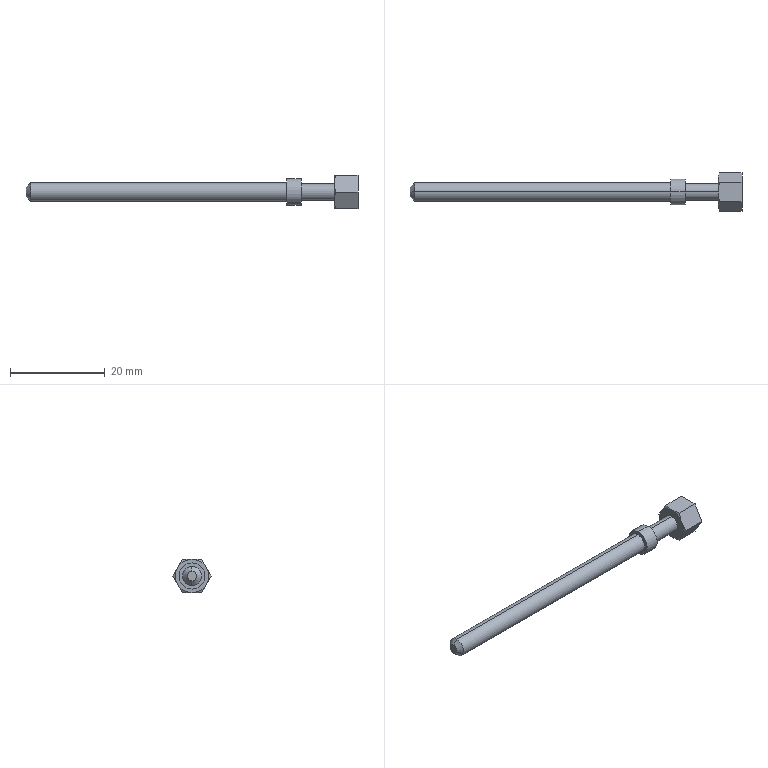Part | STEP file | 11-AJST4-5511 | 1 solid | 25 faces | box 70 x 8.083 x 7 mm | volume 1036 mm3 | plane 11 | cone 8 | cylinder 6 | commonest cylinder face diameters 3.5 x2 4 x2 5.5 x2
STEP:
#1=CARTESIAN_POINT('',(0.,0.,1.));
#2=VERTEX_POINT('',#1);
#3=CARTESIAN_POINT('',(0.,0.,-1.));
#4=VERTEX_POINT('',#3);
#5=CARTESIAN_POINT('',(0.,0.,0.));
#6=DIRECTION('',(-1.,0.,0.));
#7=DIRECTION('',(0.,0.,-1.));
#8=AXIS2_PLACEMENT_3D('',#5,#6,#7);
#9=CIRCLE('',#8,1.);
#10=EDGE_CURVE('',#2,#4,#9,.T.);
#11=ORIENTED_EDGE('',*,*,#10,.F.);
#12=CARTESIAN_POINT('',(1.,0.,2.));
#13=VERTEX_POINT('',#12);
#14=CARTESIAN_POINT('',(0.,0.,1.));
#15=DIRECTION('',(0.7071,0.,0.7071));
#16=VECTOR('',#15,1000.);
#17=LINE('',#14,#16);
#18=EDGE_CURVE('',#2,#13,#17,.T.);
#19=ORIENTED_EDGE('',*,*,#18,.T.);
#20=CARTESIAN_POINT('',(1.,0.,-2.));
#21=VERTEX_POINT('',#20);
#22=CARTESIAN_POINT('',(1.,0.,0.));
#23=DIRECTION('',(1.,0.,0.));
#24=DIRECTION('',(0.,0.,-1.));
#25=AXIS2_PLACEMENT_3D('',#22,#23,#24);
#26=CIRCLE('',#25,2.);
#27=EDGE_CURVE('',#21,#13,#26,.T.);
#28=ORIENTED_EDGE('',*,*,#27,.F.);
#29=CARTESIAN_POINT('',(0.,0.,-1.));
#30=DIRECTION('',(0.7071,0.,-0.7071));
#31=VECTOR('',#30,1000.);
#32=LINE('',#29,#31);
#33=EDGE_CURVE('',#4,#21,#32,.T.);
#34=ORIENTED_EDGE('',*,*,#33,.F.);
#35=EDGE_LOOP('',(#11,#19,#28,#34));
#36=FACE_OUTER_BOUND('',#35,.T.);
#37=CARTESIAN_POINT('',(0.,0.,0.));
#38=DIRECTION('',(1.,0.,0.));
#39=DIRECTION('',(0.,0.,-1.));
#40=AXIS2_PLACEMENT_3D('',#37,#38,#39);
#41=CONICAL_SURFACE('',#40,1.,0.7854);
#42=ADVANCED_FACE('',(#36),#41,.T.);
#43=CARTESIAN_POINT('',(65.,0.,-1.75));
#44=VERTEX_POINT('',#43);
#45=CARTESIAN_POINT('',(65.,0.,1.75));
#46=VERTEX_POINT('',#45);
#47=CARTESIAN_POINT('',(65.,0.,0.));
#48=DIRECTION('',(1.,0.,0.));
#49=DIRECTION('',(0.,0.,-1.));
#50=AXIS2_PLACEMENT_3D('',#47,#48,#49);
#51=CIRCLE('',#50,1.75);
#52=EDGE_CURVE('',#44,#46,#51,.T.);
#53=ORIENTED_EDGE('',*,*,#52,.F.);
#54=CARTESIAN_POINT('',(58.,0.,-1.75));
#55=VERTEX_POINT('',#54);
#56=CARTESIAN_POINT('',(0.,0.,-1.75));
#57=DIRECTION('',(-1.,0.,0.));
#58=VECTOR('',#57,1000.);
#59=LINE('',#56,#58);
#60=EDGE_CURVE('',#44,#55,#59,.T.);
#61=ORIENTED_EDGE('',*,*,#60,.T.);
#62=CARTESIAN_POINT('',(58.,0.,1.75));
#63=VERTEX_POINT('',#62);
#64=CARTESIAN_POINT('',(58.,0.,0.));
#65=DIRECTION('',(-1.,0.,0.));
#66=DIRECTION('',(0.,0.,1.));
#67=AXIS2_PLACEMENT_3D('',#64,#65,#66);
#68=CIRCLE('',#67,1.75);
#69=EDGE_CURVE('',#63,#55,#68,.T.);
#70=ORIENTED_EDGE('',*,*,#69,.F.);
#71=CARTESIAN_POINT('',(0.,0.,1.75));
#72=DIRECTION('',(-1.,0.,0.));
#73=VECTOR('',#72,1000.);
#74=LINE('',#71,#73);
#75=EDGE_CURVE('',#46,#63,#74,.T.);
#76=ORIENTED_EDGE('',*,*,#75,.F.);
#77=EDGE_LOOP('',(#53,#61,#70,#76));
#78=FACE_OUTER_BOUND('',#77,.T.);
#79=CARTESIAN_POINT('',(0.,0.,0.));
#80=DIRECTION('',(-1.,0.,0.));
#81=DIRECTION('',(0.,0.,1.));
#82=AXIS2_PLACEMENT_3D('',#79,#80,#81);
#83=CYLINDRICAL_SURFACE('',#82,1.75);
#84=ADVANCED_FACE('',(#78),#83,.T.);
#85=CARTESIAN_POINT('',(58.,0.,2.75));
#86=VERTEX_POINT('',#85);
#87=CARTESIAN_POINT('',(58.,0.,-2.75));
#88=VERTEX_POINT('',#87);
#89=CARTESIAN_POINT('',(58.,0.,0.));
#90=DIRECTION('',(-1.,0.,0.));
#91=DIRECTION('',(0.,0.,1.));
#92=AXIS2_PLACEMENT_3D('',#89,#90,#91);
#93=CIRCLE('',#92,2.75);
#94=EDGE_CURVE('',#86,#88,#93,.T.);
#95=ORIENTED_EDGE('',*,*,#94,.T.);
#96=CARTESIAN_POINT('',(55.,0.,-2.75));
#97=VERTEX_POINT('',#96);
#98=CARTESIAN_POINT('',(0.,0.,-2.75));
#99=DIRECTION('',(-1.,0.,0.));
#100=VECTOR('',#99,1000.);
#101=LINE('',#98,#100);
#102=EDGE_CURVE('',#88,#97,#101,.T.);
#103=ORIENTED_EDGE('',*,*,#102,.T.);
#104=CARTESIAN_POINT('',(55.,0.,2.75));
#105=VERTEX_POINT('',#104);
#106=CARTESIAN_POINT('',(55.,0.,0.));
#107=DIRECTION('',(-1.,0.,0.));
#108=DIRECTION('',(0.,0.,1.));
#109=AXIS2_PLACEMENT_3D('',#106,#107,#108);
#110=CIRCLE('',#109,2.75);
#111=EDGE_CURVE('',#105,#97,#110,.T.);
#112=ORIENTED_EDGE('',*,*,#111,.F.);
#113=CARTESIAN_POINT('',(0.,0.,2.75));
#114=DIRECTION('',(-1.,0.,0.));
#115=VECTOR('',#114,1000.);
#116=LINE('',#113,#115);
#117=EDGE_CURVE('',#86,#105,#116,.T.);
#118=ORIENTED_EDGE('',*,*,#117,.F.);
#119=EDGE_LOOP('',(#95,#103,#112,#118));
#120=FACE_OUTER_BOUND('',#119,.T.);
#121=CARTESIAN_POINT('',(0.,0.,0.));
#122=DIRECTION('',(-1.,0.,0.));
#123=DIRECTION('',(0.,0.,1.));
#124=AXIS2_PLACEMENT_3D('',#121,#122,#123);
#125=CYLINDRICAL_SURFACE('',#124,2.75);
#126=ADVANCED_FACE('',(#120),#125,.T.);
#127=CARTESIAN_POINT('',(55.,0.,2.));
#128=VERTEX_POINT('',#127);
#129=CARTESIAN_POINT('',(55.,0.,-2.));
#130=VERTEX_POINT('',#129);
#131=CARTESIAN_POINT('',(55.,0.,0.));
#132=DIRECTION('',(-1.,0.,0.));
#133=DIRECTION('',(0.,0.,1.));
#134=AXIS2_PLACEMENT_3D('',#131,#132,#133);
#135=CIRCLE('',#134,2.);
#136=EDGE_CURVE('',#128,#130,#135,.T.);
#137=ORIENTED_EDGE('',*,*,#136,.T.);
#138=CARTESIAN_POINT('',(0.,0.,-2.));
#139=DIRECTION('',(-1.,0.,0.));
#140=VECTOR('',#139,1000.);
#141=LINE('',#138,#140);
#142=EDGE_CURVE('',#130,#21,#141,.T.);
#143=ORIENTED_EDGE('',*,*,#142,.T.);
#144=ORIENTED_EDGE('',*,*,#27,.T.);
#145=CARTESIAN_POINT('',(0.,0.,2.));
#146=DIRECTION('',(-1.,0.,0.));
#147=VECTOR('',#146,1000.);
#148=LINE('',#145,#147);
#149=EDGE_CURVE('',#128,#13,#148,.T.);
#150=ORIENTED_EDGE('',*,*,#149,.F.);
#151=EDGE_LOOP('',(#137,#143,#144,#150));
#152=FACE_OUTER_BOUND('',#151,.T.);
#153=CARTESIAN_POINT('',(0.,0.,0.));
#154=DIRECTION('',(-1.,0.,0.));
#155=DIRECTION('',(0.,0.,1.));
#156=AXIS2_PLACEMENT_3D('',#153,#154,#155);
#157=CYLINDRICAL_SURFACE('',#156,2.);
#158=ADVANCED_FACE('',(#152),#157,.T.);
#159=CARTESIAN_POINT('',(65.,0.,0.));
#160=DIRECTION('',(1.,0.,0.));
#161=DIRECTION('',(0.,0.,-1.));
#162=AXIS2_PLACEMENT_3D('',#159,#160,#161);
#163=CIRCLE('',#162,1.75);
#164=EDGE_CURVE('',#46,#44,#163,.T.);
#165=ORIENTED_EDGE('',*,*,#164,.T.);
#166=ORIENTED_EDGE('',*,*,#52,.T.);
#167=EDGE_LOOP('',(#165,#166));
#168=FACE_BOUND('',#167,.T.);
#169=CARTESIAN_POINT('',(65.,3.031,-1.75));
#170=VERTEX_POINT('',#169);
#171=CARTESIAN_POINT('',(65.,0.,-3.5));
#172=VERTEX_POINT('',#171);
#173=CARTESIAN_POINT('',(65.,0.,0.));
#174=DIRECTION('',(-1.,0.,0.));
#175=DIRECTION('',(0.,0.,1.));
#176=AXIS2_PLACEMENT_3D('',#173,#174,#175);
#177=CIRCLE('',#176,3.5);
#178=EDGE_CURVE('',#170,#172,#177,.T.);
#179=ORIENTED_EDGE('',*,*,#178,.T.);
#180=CARTESIAN_POINT('',(65.,-3.031,-1.75));
#181=VERTEX_POINT('',#180);
#182=CARTESIAN_POINT('',(65.,0.,0.));
#183=DIRECTION('',(-1.,0.,0.));
#184=DIRECTION('',(0.,0.,1.));
#185=AXIS2_PLACEMENT_3D('',#182,#183,#184);
#186=CIRCLE('',#185,3.5);
#187=EDGE_CURVE('',#172,#181,#186,.T.);
#188=ORIENTED_EDGE('',*,*,#187,.T.);
#189=CARTESIAN_POINT('',(65.,-3.031,1.75));
#190=VERTEX_POINT('',#189);
#191=CARTESIAN_POINT('',(65.,0.,0.));
#192=DIRECTION('',(-1.,0.,0.));
#193=DIRECTION('',(0.,0.,1.));
#194=AXIS2_PLACEMENT_3D('',#191,#192,#193);
#195=CIRCLE('',#194,3.5);
#196=EDGE_CURVE('',#181,#190,#195,.T.);
#197=ORIENTED_EDGE('',*,*,#196,.T.);
#198=CARTESIAN_POINT('',(65.,0.,3.5));
#199=VERTEX_POINT('',#198);
#200=CARTESIAN_POINT('',(65.,0.,0.));
#201=DIRECTION('',(-1.,0.,0.));
#202=DIRECTION('',(0.,0.,1.));
#203=AXIS2_PLACEMENT_3D('',#200,#201,#202);
#204=CIRCLE('',#203,3.5);
#205=EDGE_CURVE('',#190,#199,#204,.T.);
#206=ORIENTED_EDGE('',*,*,#205,.T.);
#207=CARTESIAN_POINT('',(65.,3.031,1.75));
#208=VERTEX_POINT('',#207);
#209=CARTESIAN_POINT('',(65.,0.,0.));
#210=DIRECTION('',(-1.,0.,0.));
#211=DIRECTION('',(0.,0.,1.));
#212=AXIS2_PLACEMENT_3D('',#209,#210,#211);
#213=CIRCLE('',#212,3.5);
#214=EDGE_CURVE('',#199,#208,#213,.T.);
#215=ORIENTED_EDGE('',*,*,#214,.T.);
#216=CARTESIAN_POINT('',(65.,0.,0.));
#217=DIRECTION('',(-1.,0.,0.));
#218=DIRECTION('',(0.,0.,1.));
#219=AXIS2_PLACEMENT_3D('',#216,#217,#218);
#220=CIRCLE('',#219,3.5);
#221=EDGE_CURVE('',#208,#170,#220,.T.);
#222=ORIENTED_EDGE('',*,*,#221,.T.);
#223=EDGE_LOOP('',(#179,#188,#197,#206,#215,#222));
#224=FACE_OUTER_BOUND('',#223,.T.);
#225=CARTESIAN_POINT('',(65.,0.,0.));
#226=DIRECTION('',(1.,0.,0.));
#227=DIRECTION('',(0.,0.,-1.));
#228=AXIS2_PLACEMENT_3D('',#225,#226,#227);
#229=PLANE('',#228);
#230=ADVANCED_FACE('',(#168,#224),#229,.F.);
#231=CARTESIAN_POINT('',(0.,0.,0.));
#232=DIRECTION('',(-1.,0.,0.));
#233=DIRECTION('',(0.,0.,-1.));
#234=AXIS2_PLACEMENT_3D('',#231,#232,#233);
#235=CIRCLE('',#234,1.);
#236=EDGE_CURVE('',#4,#2,#235,.T.);
#237=ORIENTED_EDGE('',*,*,#236,.T.);
#238=ORIENTED_EDGE('',*,*,#10,.T.);
#239=EDGE_LOOP('',(#237,#238));
#240=FACE_OUTER_BOUND('',#239,.T.);
#241=CARTESIAN_POINT('',(0.,0.,0.));
#242=DIRECTION('',(1.,0.,0.));
#243=DIRECTION('',(0.,0.,-1.));
#244=AXIS2_PLACEMENT_3D('',#241,#242,#243);
#245=PLANE('',#244);
#246=ADVANCED_FACE('',(#240),#245,.F.);
#247=ORIENTED_EDGE('',*,*,#142,.F.);
#248=CARTESIAN_POINT('',(55.,0.,0.));
#249=DIRECTION('',(-1.,0.,0.));
#250=DIRECTION('',(0.,0.,1.));
#251=AXIS2_PLACEMENT_3D('',#248,#249,#250);
#252=CIRCLE('',#251,2.);
#253=EDGE_CURVE('',#130,#128,#252,.T.);
#254=ORIENTED_EDGE('',*,*,#253,.T.);
#255=ORIENTED_EDGE('',*,*,#149,.T.);
#256=CARTESIAN_POINT('',(1.,0.,0.));
#257=DIRECTION('',(1.,0.,0.));
#258=DIRECTION('',(0.,0.,-1.));
#259=AXIS2_PLACEMENT_3D('',#256,#257,#258);
#260=CIRCLE('',#259,2.);
#261=EDGE_CURVE('',#13,#21,#260,.T.);
#262=ORIENTED_EDGE('',*,*,#261,.T.);
#263=EDGE_LOOP('',(#247,#254,#255,#262));
#264=FACE_OUTER_BOUND('',#263,.T.);
#265=CARTESIAN_POINT('',(0.,0.,0.));
#266=DIRECTION('',(-1.,0.,0.));
#267=DIRECTION('',(0.,0.,1.));
#268=AXIS2_PLACEMENT_3D('',#265,#266,#267);
#269=CYLINDRICAL_SURFACE('',#268,2.);
#270=ADVANCED_FACE('',(#264),#269,.T.);
#271=ORIENTED_EDGE('',*,*,#136,.F.);
#272=ORIENTED_EDGE('',*,*,#253,.F.);
#273=EDGE_LOOP('',(#271,#272));
#274=FACE_BOUND('',#273,.T.);
#275=ORIENTED_EDGE('',*,*,#111,.T.);
#276=CARTESIAN_POINT('',(55.,0.,0.));
#277=DIRECTION('',(-1.,0.,0.));
#278=DIRECTION('',(0.,0.,1.));
#279=AXIS2_PLACEMENT_3D('',#276,#277,#278);
#280=CIRCLE('',#279,2.75);
#281=EDGE_CURVE('',#97,#105,#280,.T.);
#282=ORIENTED_EDGE('',*,*,#281,.T.);
#283=EDGE_LOOP('',(#275,#282));
#284=FACE_OUTER_BOUND('',#283,.T.);
#285=CARTESIAN_POINT('',(55.,2.,0.));
#286=DIRECTION('',(1.,0.,0.));
#287=DIRECTION('',(0.,0.,-1.));
#288=AXIS2_PLACEMENT_3D('',#285,#286,#287);
#289=PLANE('',#288);
#290=ADVANCED_FACE('',(#274,#284),#289,.F.);
#291=ORIENTED_EDGE('',*,*,#102,.F.);
#292=CARTESIAN_POINT('',(58.,0.,0.));
#293=DIRECTION('',(-1.,0.,0.));
#294=DIRECTION('',(0.,0.,1.));
#295=AXIS2_PLACEMENT_3D('',#292,#293,#294);
#296=CIRCLE('',#295,2.75);
#297=EDGE_CURVE('',#88,#86,#296,.T.);
#298=ORIENTED_EDGE('',*,*,#297,.T.);
#299=ORIENTED_EDGE('',*,*,#117,.T.);
#300=ORIENTED_EDGE('',*,*,#281,.F.);
#301=EDGE_LOOP('',(#291,#298,#299,#300));
#302=FACE_OUTER_BOUND('',#301,.T.);
#303=CARTESIAN_POINT('',(0.,0.,0.));
#304=DIRECTION('',(-1.,0.,0.));
#305=DIRECTION('',(0.,0.,1.));
#306=AXIS2_PLACEMENT_3D('',#303,#304,#305);
#307=CYLINDRICAL_SURFACE('',#306,2.75);
#308=ADVANCED_FACE('',(#302),#307,.T.);
#309=ORIENTED_EDGE('',*,*,#94,.F.);
#310=ORIENTED_EDGE('',*,*,#297,.F.);
#311=EDGE_LOOP('',(#309,#310));
#312=FACE_OUTER_BOUND('',#311,.T.);
#313=ORIENTED_EDGE('',*,*,#69,.T.);
#314=CARTESIAN_POINT('',(58.,0.,0.));
#315=DIRECTION('',(-1.,0.,0.));
#316=DIRECTION('',(0.,0.,1.));
#317=AXIS2_PLACEMENT_3D('',#314,#315,#316);
#318=CIRCLE('',#317,1.75);
#319=EDGE_CURVE('',#55,#63,#318,.T.);
#320=ORIENTED_EDGE('',*,*,#319,.T.);
#321=EDGE_LOOP('',(#313,#320));
#322=FACE_BOUND('',#321,.T.);
#323=CARTESIAN_POINT('',(58.,2.75,0.));
#324=DIRECTION('',(-1.,0.,0.));
#325=DIRECTION('',(0.,0.,1.));
#326=AXIS2_PLACEMENT_3D('',#323,#324,#325);
#327=PLANE('',#326);
#328=ADVANCED_FACE('',(#312,#322),#327,.F.);
#329=ORIENTED_EDGE('',*,*,#60,.F.);
#330=ORIENTED_EDGE('',*,*,#164,.F.);
#331=ORIENTED_EDGE('',*,*,#75,.T.);
#332=ORIENTED_EDGE('',*,*,#319,.F.);
#333=EDGE_LOOP('',(#329,#330,#331,#332));
#334=FACE_OUTER_BOUND('',#333,.T.);
#335=CARTESIAN_POINT('',(0.,0.,0.));
#336=DIRECTION('',(-1.,0.,0.));
#337=DIRECTION('',(0.,0.,1.));
#338=AXIS2_PLACEMENT_3D('',#335,#336,#337);
#339=CYLINDRICAL_SURFACE('',#338,1.75);
#340=ADVANCED_FACE('',(#334),#339,.T.);
#341=CARTESIAN_POINT('',(65.313,-2.021,3.5));
#342=VERTEX_POINT('',#341);
#343=CARTESIAN_POINT('',(65.313,-2.021,3.5));
#344=CARTESIAN_POINT('',(65.218,-1.692,3.5));
#345=CARTESIAN_POINT('',(65.138,-1.355,3.5));
#346=CARTESIAN_POINT('',(65.029,-0.6807,3.5));
#347=CARTESIAN_POINT('',(65.,-0.3415,3.5));
#348=CARTESIAN_POINT('',(65.,0.,3.5));
#349=B_SPLINE_CURVE_WITH_KNOTS('',3,(#343,#344,#345,#346,#347,#348),.UNSPECIFIED.,.F.,.F.,(4,2,4),(0.003605,0.004627,0.005649),.UNSPECIFIED.);
#350=EDGE_CURVE('',#342,#199,#349,.T.);
#351=ORIENTED_EDGE('',*,*,#350,.T.);
#352=ORIENTED_EDGE('',*,*,#205,.F.);
#353=CARTESIAN_POINT('',(65.,-3.031,1.75));
#354=CARTESIAN_POINT('',(65.,-2.86,2.047));
#355=CARTESIAN_POINT('',(65.03,-2.688,2.344));
#356=CARTESIAN_POINT('',(65.139,-2.352,2.926));
#357=CARTESIAN_POINT('',(65.217,-2.186,3.214));
#358=CARTESIAN_POINT('',(65.313,-2.021,3.5));
#359=B_SPLINE_CURVE_WITH_KNOTS('',3,(#353,#354,#355,#356,#357,#358),.UNSPECIFIED.,.F.,.F.,(4,2,4),(0.002045,0.003063,0.004082),.UNSPECIFIED.);
#360=EDGE_CURVE('',#190,#342,#359,.T.);
#361=ORIENTED_EDGE('',*,*,#360,.T.);
#362=EDGE_LOOP('',(#351,#352,#361));
#363=FACE_OUTER_BOUND('',#362,.T.);
#364=CARTESIAN_POINT('',(65.,0.,0.));
#365=DIRECTION('',(1.,0.,0.));
#366=DIRECTION('',(0.,0.,-1.));
#367=AXIS2_PLACEMENT_3D('',#364,#365,#366);
#368=CONICAL_SURFACE('',#367,3.5,1.047);
#369=ADVANCED_FACE('',(#363),#368,.T.);
#370=CARTESIAN_POINT('',(65.313,-4.041,0.));
#371=VERTEX_POINT('',#370);
#372=CARTESIAN_POINT('',(65.,-3.031,-1.75));
#373=CARTESIAN_POINT('',(65.,-3.203,-1.453));
#374=CARTESIAN_POINT('',(65.03,-3.374,-1.156));
#375=CARTESIAN_POINT('',(65.139,-3.71,-0.5735));
#376=CARTESIAN_POINT('',(65.217,-3.877,-0.2856));
#377=CARTESIAN_POINT('',(65.313,-4.041,0.));
#378=B_SPLINE_CURVE_WITH_KNOTS('',3,(#372,#373,#374,#375,#376,#377),.UNSPECIFIED.,.F.,.F.,(4,2,4),(0.002045,0.003063,0.004082),.UNSPECIFIED.);
#379=EDGE_CURVE('',#181,#371,#378,.T.);
#380=ORIENTED_EDGE('',*,*,#379,.T.);
#381=CARTESIAN_POINT('',(65.313,-4.041,0.));
#382=CARTESIAN_POINT('',(65.122,-3.711,0.5726));
#383=CARTESIAN_POINT('',(65.,-3.375,1.154));
#384=CARTESIAN_POINT('',(65.,-3.031,1.75));
#385=B_SPLINE_CURVE_WITH_KNOTS('',3,(#381,#382,#383,#384),.UNSPECIFIED.,.F.,.F.,(4,4),(0.000000238,0.002045),.UNSPECIFIED.);
#386=EDGE_CURVE('',#371,#190,#385,.T.);
#387=ORIENTED_EDGE('',*,*,#386,.T.);
#388=ORIENTED_EDGE('',*,*,#196,.F.);
#389=EDGE_LOOP('',(#380,#387,#388));
#390=FACE_OUTER_BOUND('',#389,.T.);
#391=CARTESIAN_POINT('',(65.,0.,0.));
#392=DIRECTION('',(1.,0.,0.));
#393=DIRECTION('',(0.,0.,-1.));
#394=AXIS2_PLACEMENT_3D('',#391,#392,#393);
#395=CONICAL_SURFACE('',#394,3.5,1.047);
#396=ADVANCED_FACE('',(#390),#395,.T.);
#397=CARTESIAN_POINT('',(65.313,2.021,3.5));
#398=VERTEX_POINT('',#397);
#399=CARTESIAN_POINT('',(65.313,2.021,3.5));
#400=CARTESIAN_POINT('',(65.122,2.351,2.927));
#401=CARTESIAN_POINT('',(65.,2.687,2.346));
#402=CARTESIAN_POINT('',(65.,3.031,1.75));
#403=B_SPLINE_CURVE_WITH_KNOTS('',3,(#399,#400,#401,#402),.UNSPECIFIED.,.F.,.F.,(4,4),(0.000000238,0.002045),.UNSPECIFIED.);
#404=EDGE_CURVE('',#398,#208,#403,.T.);
#405=ORIENTED_EDGE('',*,*,#404,.T.);
#406=ORIENTED_EDGE('',*,*,#214,.F.);
#407=CARTESIAN_POINT('',(65.,0.,3.5));
#408=CARTESIAN_POINT('',(65.,0.3417,3.5));
#409=CARTESIAN_POINT('',(65.03,0.688,3.5));
#410=CARTESIAN_POINT('',(65.14,1.363,3.5));
#411=CARTESIAN_POINT('',(65.218,1.694,3.5));
#412=CARTESIAN_POINT('',(65.313,2.021,3.5));
#413=B_SPLINE_CURVE_WITH_KNOTS('',3,(#407,#408,#409,#410,#411,#412),.UNSPECIFIED.,.F.,.F.,(4,2,4),(0.005649,0.006672,0.007695),.UNSPECIFIED.);
#414=EDGE_CURVE('',#199,#398,#413,.T.);
#415=ORIENTED_EDGE('',*,*,#414,.T.);
#416=EDGE_LOOP('',(#405,#406,#415));
#417=FACE_OUTER_BOUND('',#416,.T.);
#418=CARTESIAN_POINT('',(65.,0.,0.));
#419=DIRECTION('',(1.,0.,0.));
#420=DIRECTION('',(0.,0.,-1.));
#421=AXIS2_PLACEMENT_3D('',#418,#419,#420);
#422=CONICAL_SURFACE('',#421,3.5,1.047);
#423=ADVANCED_FACE('',(#417),#422,.T.);
#424=CARTESIAN_POINT('',(65.313,4.041,0.));
#425=VERTEX_POINT('',#424);
#426=CARTESIAN_POINT('',(65.313,4.041,0.));
#427=CARTESIAN_POINT('',(65.122,3.711,-0.5726));
#428=CARTESIAN_POINT('',(65.,3.375,-1.154));
#429=CARTESIAN_POINT('',(65.,3.031,-1.75));
#430=B_SPLINE_CURVE_WITH_KNOTS('',3,(#426,#427,#428,#429),.UNSPECIFIED.,.F.,.F.,(4,4),(0.000000238,0.002045),.UNSPECIFIED.);
#431=EDGE_CURVE('',#425,#170,#430,.T.);
#432=ORIENTED_EDGE('',*,*,#431,.T.);
#433=ORIENTED_EDGE('',*,*,#221,.F.);
#434=CARTESIAN_POINT('',(65.,3.031,1.75));
#435=CARTESIAN_POINT('',(65.,3.203,1.453));
#436=CARTESIAN_POINT('',(65.03,3.374,1.156));
#437=CARTESIAN_POINT('',(65.139,3.71,0.5735));
#438=CARTESIAN_POINT('',(65.217,3.877,0.2856));
#439=CARTESIAN_POINT('',(65.313,4.041,0.));
#440=B_SPLINE_CURVE_WITH_KNOTS('',3,(#434,#435,#436,#437,#438,#439),.UNSPECIFIED.,.F.,.F.,(4,2,4),(0.002045,0.003063,0.004082),.UNSPECIFIED.);
#441=EDGE_CURVE('',#208,#425,#440,.T.);
#442=ORIENTED_EDGE('',*,*,#441,.T.);
#443=EDGE_LOOP('',(#432,#433,#442));
#444=FACE_OUTER_BOUND('',#443,.T.);
#445=CARTESIAN_POINT('',(65.,0.,0.));
#446=DIRECTION('',(1.,0.,0.));
#447=DIRECTION('',(0.,0.,-1.));
#448=AXIS2_PLACEMENT_3D('',#445,#446,#447);
#449=CONICAL_SURFACE('',#448,3.5,1.047);
#450=ADVANCED_FACE('',(#444),#449,.T.);
#451=CARTESIAN_POINT('',(65.313,2.021,-3.5));
#452=VERTEX_POINT('',#451);
#453=CARTESIAN_POINT('',(65.,3.031,-1.75));
#454=CARTESIAN_POINT('',(65.,2.86,-2.047));
#455=CARTESIAN_POINT('',(65.03,2.688,-2.344));
#456=CARTESIAN_POINT('',(65.139,2.352,-2.926));
#457=CARTESIAN_POINT('',(65.217,2.186,-3.214));
#458=CARTESIAN_POINT('',(65.313,2.021,-3.5));
#459=B_SPLINE_CURVE_WITH_KNOTS('',3,(#453,#454,#455,#456,#457,#458),.UNSPECIFIED.,.F.,.F.,(4,2,4),(0.002045,0.003063,0.004082),.UNSPECIFIED.);
#460=EDGE_CURVE('',#170,#452,#459,.T.);
#461=ORIENTED_EDGE('',*,*,#460,.T.);
#462=CARTESIAN_POINT('',(65.313,2.021,-3.5));
#463=CARTESIAN_POINT('',(65.218,1.694,-3.5));
#464=CARTESIAN_POINT('',(65.14,1.363,-3.5));
#465=CARTESIAN_POINT('',(65.03,0.688,-3.5));
#466=CARTESIAN_POINT('',(65.,0.3417,-3.5));
#467=CARTESIAN_POINT('',(65.,0.,-3.5));
#468=B_SPLINE_CURVE_WITH_KNOTS('',3,(#462,#463,#464,#465,#466,#467),.UNSPECIFIED.,.F.,.F.,(4,2,4),(0.001481,0.002501,0.003521),.UNSPECIFIED.);
#469=EDGE_CURVE('',#452,#172,#468,.T.);
#470=ORIENTED_EDGE('',*,*,#469,.T.);
#471=ORIENTED_EDGE('',*,*,#178,.F.);
#472=EDGE_LOOP('',(#461,#470,#471));
#473=FACE_OUTER_BOUND('',#472,.T.);
#474=CARTESIAN_POINT('',(65.,0.,0.));
#475=DIRECTION('',(1.,0.,0.));
#476=DIRECTION('',(0.,0.,-1.));
#477=AXIS2_PLACEMENT_3D('',#474,#475,#476);
#478=CONICAL_SURFACE('',#477,3.5,1.047);
#479=ADVANCED_FACE('',(#473),#478,.T.);
#480=CARTESIAN_POINT('',(65.313,-2.021,-3.5));
#481=VERTEX_POINT('',#480);
#482=CARTESIAN_POINT('',(65.,0.,-3.5));
#483=CARTESIAN_POINT('',(65.,-0.3415,-3.5));
#484=CARTESIAN_POINT('',(65.029,-0.6807,-3.5));
#485=CARTESIAN_POINT('',(65.138,-1.355,-3.5));
#486=CARTESIAN_POINT('',(65.218,-1.692,-3.5));
#487=CARTESIAN_POINT('',(65.313,-2.021,-3.5));
#488=B_SPLINE_CURVE_WITH_KNOTS('',3,(#482,#483,#484,#485,#486,#487),.UNSPECIFIED.,.F.,.F.,(4,2,4),(0.003521,0.004541,0.005561),.UNSPECIFIED.);
#489=EDGE_CURVE('',#172,#481,#488,.T.);
#490=ORIENTED_EDGE('',*,*,#489,.T.);
#491=CARTESIAN_POINT('',(65.313,-2.021,-3.5));
#492=CARTESIAN_POINT('',(65.122,-2.351,-2.927));
#493=CARTESIAN_POINT('',(65.,-2.687,-2.346));
#494=CARTESIAN_POINT('',(65.,-3.031,-1.75));
#495=B_SPLINE_CURVE_WITH_KNOTS('',3,(#491,#492,#493,#494),.UNSPECIFIED.,.F.,.F.,(4,4),(0.000000238,0.002045),.UNSPECIFIED.);
#496=EDGE_CURVE('',#481,#181,#495,.T.);
#497=ORIENTED_EDGE('',*,*,#496,.T.);
#498=ORIENTED_EDGE('',*,*,#187,.F.);
#499=EDGE_LOOP('',(#490,#497,#498));
#500=FACE_OUTER_BOUND('',#499,.T.);
#501=CARTESIAN_POINT('',(65.,0.,0.));
#502=DIRECTION('',(1.,0.,0.));
#503=DIRECTION('',(0.,0.,-1.));
#504=AXIS2_PLACEMENT_3D('',#501,#502,#503);
#505=CONICAL_SURFACE('',#504,3.5,1.047);
#506=ADVANCED_FACE('',(#500),#505,.T.);
#507=CARTESIAN_POINT('',(70.,-4.041,0.));
#508=VERTEX_POINT('',#507);
#509=CARTESIAN_POINT('',(70.,-2.021,-3.5));
#510=VERTEX_POINT('',#509);
#511=CARTESIAN_POINT('',(70.,-4.041,0.));
#512=DIRECTION('',(0.,0.5,-0.866));
#513=VECTOR('',#512,1000.);
#514=LINE('',#511,#513);
#515=EDGE_CURVE('',#508,#510,#514,.T.);
#516=ORIENTED_EDGE('',*,*,#515,.T.);
#517=CARTESIAN_POINT('',(70.,2.021,-3.5));
#518=VERTEX_POINT('',#517);
#519=CARTESIAN_POINT('',(70.,-2.021,-3.5));
#520=DIRECTION('',(0.,1.,0.));
#521=VECTOR('',#520,1000.);
#522=LINE('',#519,#521);
#523=EDGE_CURVE('',#510,#518,#522,.T.);
#524=ORIENTED_EDGE('',*,*,#523,.T.);
#525=CARTESIAN_POINT('',(70.,4.041,0.));
#526=VERTEX_POINT('',#525);
#527=CARTESIAN_POINT('',(70.,2.021,-3.5));
#528=DIRECTION('',(0.,0.5,0.866));
#529=VECTOR('',#528,1000.);
#530=LINE('',#527,#529);
#531=EDGE_CURVE('',#518,#526,#530,.T.);
#532=ORIENTED_EDGE('',*,*,#531,.T.);
#533=CARTESIAN_POINT('',(70.,2.021,3.5));
#534=VERTEX_POINT('',#533);
#535=CARTESIAN_POINT('',(70.,4.041,0.));
#536=DIRECTION('',(0.,-0.5,0.866));
#537=VECTOR('',#536,1000.);
#538=LINE('',#535,#537);
#539=EDGE_CURVE('',#526,#534,#538,.T.);
#540=ORIENTED_EDGE('',*,*,#539,.T.);
#541=CARTESIAN_POINT('',(70.,-2.021,3.5));
#542=VERTEX_POINT('',#541);
#543=CARTESIAN_POINT('',(70.,2.021,3.5));
#544=DIRECTION('',(0.,-1.,0.));
#545=VECTOR('',#544,1000.);
#546=LINE('',#543,#545);
#547=EDGE_CURVE('',#534,#542,#546,.T.);
#548=ORIENTED_EDGE('',*,*,#547,.T.);
#549=CARTESIAN_POINT('',(70.,-2.021,3.5));
#550=DIRECTION('',(0.,-0.5,-0.866));
#551=VECTOR('',#550,1000.);
#552=LINE('',#549,#551);
#553=EDGE_CURVE('',#542,#508,#552,.T.);
#554=ORIENTED_EDGE('',*,*,#553,.T.);
#555=EDGE_LOOP('',(#516,#524,#532,#540,#548,#554));
#556=FACE_OUTER_BOUND('',#555,.T.);
#557=CARTESIAN_POINT('',(70.,0.,0.));
#558=DIRECTION('',(1.,0.,0.));
#559=DIRECTION('',(0.,0.,-1.));
#560=AXIS2_PLACEMENT_3D('',#557,#558,#559);
#561=PLANE('',#560);
#562=ADVANCED_FACE('',(#556),#561,.T.);
#563=ORIENTED_EDGE('',*,*,#386,.F.);
#564=CARTESIAN_POINT('',(70.,-4.041,0.));
#565=DIRECTION('',(-1.,0.,0.));
#566=VECTOR('',#565,1000.);
#567=LINE('',#564,#566);
#568=EDGE_CURVE('',#508,#371,#567,.T.);
#569=ORIENTED_EDGE('',*,*,#568,.F.);
#570=ORIENTED_EDGE('',*,*,#553,.F.);
#571=CARTESIAN_POINT('',(70.,-2.021,3.5));
#572=DIRECTION('',(-1.,0.,0.));
#573=VECTOR('',#572,1000.);
#574=LINE('',#571,#573);
#575=EDGE_CURVE('',#542,#342,#574,.T.);
#576=ORIENTED_EDGE('',*,*,#575,.T.);
#577=ORIENTED_EDGE('',*,*,#360,.F.);
#578=EDGE_LOOP('',(#563,#569,#570,#576,#577));
#579=FACE_OUTER_BOUND('',#578,.T.);
#580=CARTESIAN_POINT('',(70.,-2.021,3.5));
#581=DIRECTION('',(0.,0.866,-0.5));
#582=DIRECTION('',(0.,0.5,0.866));
#583=AXIS2_PLACEMENT_3D('',#580,#581,#582);
#584=PLANE('',#583);
#585=ADVANCED_FACE('',(#579),#584,.F.);
#586=ORIENTED_EDGE('',*,*,#350,.F.);
#587=ORIENTED_EDGE('',*,*,#575,.F.);
#588=ORIENTED_EDGE('',*,*,#547,.F.);
#589=CARTESIAN_POINT('',(70.,2.021,3.5));
#590=DIRECTION('',(-1.,0.,0.));
#591=VECTOR('',#590,1000.);
#592=LINE('',#589,#591);
#593=EDGE_CURVE('',#534,#398,#592,.T.);
#594=ORIENTED_EDGE('',*,*,#593,.T.);
#595=ORIENTED_EDGE('',*,*,#414,.F.);
#596=EDGE_LOOP('',(#586,#587,#588,#594,#595));
#597=FACE_OUTER_BOUND('',#596,.T.);
#598=CARTESIAN_POINT('',(70.,2.021,3.5));
#599=DIRECTION('',(0.,0.,-1.));
#600=DIRECTION('',(-1.,0.,0.));
#601=AXIS2_PLACEMENT_3D('',#598,#599,#600);
#602=PLANE('',#601);
#603=ADVANCED_FACE('',(#597),#602,.F.);
#604=ORIENTED_EDGE('',*,*,#404,.F.);
#605=ORIENTED_EDGE('',*,*,#593,.F.);
#606=ORIENTED_EDGE('',*,*,#539,.F.);
#607=CARTESIAN_POINT('',(70.,4.041,0.));
#608=DIRECTION('',(-1.,0.,0.));
#609=VECTOR('',#608,1000.);
#610=LINE('',#607,#609);
#611=EDGE_CURVE('',#526,#425,#610,.T.);
#612=ORIENTED_EDGE('',*,*,#611,.T.);
#613=ORIENTED_EDGE('',*,*,#441,.F.);
#614=EDGE_LOOP('',(#604,#605,#606,#612,#613));
#615=FACE_OUTER_BOUND('',#614,.T.);
#616=CARTESIAN_POINT('',(70.,4.041,0.));
#617=DIRECTION('',(0.,-0.866,-0.5));
#618=DIRECTION('',(0.,0.5,-0.866));
#619=AXIS2_PLACEMENT_3D('',#616,#617,#618);
#620=PLANE('',#619);
#621=ADVANCED_FACE('',(#615),#620,.F.);
#622=ORIENTED_EDGE('',*,*,#431,.F.);
#623=ORIENTED_EDGE('',*,*,#611,.F.);
#624=ORIENTED_EDGE('',*,*,#531,.F.);
#625=CARTESIAN_POINT('',(70.,2.021,-3.5));
#626=DIRECTION('',(-1.,0.,0.));
#627=VECTOR('',#626,1000.);
#628=LINE('',#625,#627);
#629=EDGE_CURVE('',#518,#452,#628,.T.);
#630=ORIENTED_EDGE('',*,*,#629,.T.);
#631=ORIENTED_EDGE('',*,*,#460,.F.);
#632=EDGE_LOOP('',(#622,#623,#624,#630,#631));
#633=FACE_OUTER_BOUND('',#632,.T.);
#634=CARTESIAN_POINT('',(70.,2.021,-3.5));
#635=DIRECTION('',(0.,-0.866,0.5));
#636=DIRECTION('',(0.,-0.5,-0.866));
#637=AXIS2_PLACEMENT_3D('',#634,#635,#636);
#638=PLANE('',#637);
#639=ADVANCED_FACE('',(#633),#638,.F.);
#640=ORIENTED_EDGE('',*,*,#469,.F.);
#641=ORIENTED_EDGE('',*,*,#629,.F.);
#642=ORIENTED_EDGE('',*,*,#523,.F.);
#643=CARTESIAN_POINT('',(70.,-2.021,-3.5));
#644=DIRECTION('',(-1.,0.,0.));
#645=VECTOR('',#644,1000.);
#646=LINE('',#643,#645);
#647=EDGE_CURVE('',#510,#481,#646,.T.);
#648=ORIENTED_EDGE('',*,*,#647,.T.);
#649=ORIENTED_EDGE('',*,*,#489,.F.);
#650=EDGE_LOOP('',(#640,#641,#642,#648,#649));
#651=FACE_OUTER_BOUND('',#650,.T.);
#652=CARTESIAN_POINT('',(70.,-2.021,-3.5));
#653=DIRECTION('',(0.,0.,1.));
#654=DIRECTION('',(1.,0.,0.));
#655=AXIS2_PLACEMENT_3D('',#652,#653,#654);
#656=PLANE('',#655);
#657=ADVANCED_FACE('',(#651),#656,.F.);
#658=ORIENTED_EDGE('',*,*,#496,.F.);
#659=ORIENTED_EDGE('',*,*,#647,.F.);
#660=ORIENTED_EDGE('',*,*,#515,.F.);
#661=ORIENTED_EDGE('',*,*,#568,.T.);
#662=ORIENTED_EDGE('',*,*,#379,.F.);
#663=EDGE_LOOP('',(#658,#659,#660,#661,#662));
#664=FACE_OUTER_BOUND('',#663,.T.);
#665=CARTESIAN_POINT('',(70.,-4.041,0.));
#666=DIRECTION('',(0.,0.866,0.5));
#667=DIRECTION('',(0.,-0.5,0.866));
#668=AXIS2_PLACEMENT_3D('',#665,#666,#667);
#669=PLANE('',#668);
#670=ADVANCED_FACE('',(#664),#669,.F.);
#671=ORIENTED_EDGE('',*,*,#18,.F.);
#672=ORIENTED_EDGE('',*,*,#236,.F.);
#673=ORIENTED_EDGE('',*,*,#33,.T.);
#674=ORIENTED_EDGE('',*,*,#261,.F.);
#675=EDGE_LOOP('',(#671,#672,#673,#674));
#676=FACE_OUTER_BOUND('',#675,.T.);
#677=CARTESIAN_POINT('',(0.,0.,0.));
#678=DIRECTION('',(1.,0.,0.));
#679=DIRECTION('',(0.,0.,-1.));
#680=AXIS2_PLACEMENT_3D('',#677,#678,#679);
#681=CONICAL_SURFACE('',#680,1.,0.7854);
#682=ADVANCED_FACE('',(#676),#681,.T.);
#683=CLOSED_SHELL('',(#42,#84,#126,#158,#230,#246,#270,#290,#308,#328,#340,#369,#396,#423,#450,#479,#506,#562,#585,#603,#621,#639,#657,#670,#682));
#684=MANIFOLD_SOLID_BREP('',#683);
#685=CARTESIAN_POINT('',(0.,0.,0.));
#686=DIRECTION('',(0.,0.,1.));
#687=DIRECTION('',(1.,0.,0.));
#688=AXIS2_PLACEMENT_3D('',#685,#686,#687);
#689=(LENGTH_UNIT()NAMED_UNIT(*)SI_UNIT(.MILLI.,.METRE.));
#690=UNCERTAINTY_MEASURE_WITH_UNIT(LENGTH_MEASURE(0.00001),#689,'','');
#691=(NAMED_UNIT(*)PLANE_ANGLE_UNIT()SI_UNIT($,.RADIAN.));
#692=(NAMED_UNIT(*)SI_UNIT($,.STERADIAN.)SOLID_ANGLE_UNIT());
#693=(GEOMETRIC_REPRESENTATION_CONTEXT(3)GLOBAL_UNCERTAINTY_ASSIGNED_CONTEXT((#690))GLOBAL_UNIT_ASSIGNED_CONTEXT((#689,#691,#692))REPRESENTATION_CONTEXT('',''));
#694=ADVANCED_BREP_SHAPE_REPRESENTATION('',(#684,#688),#693);